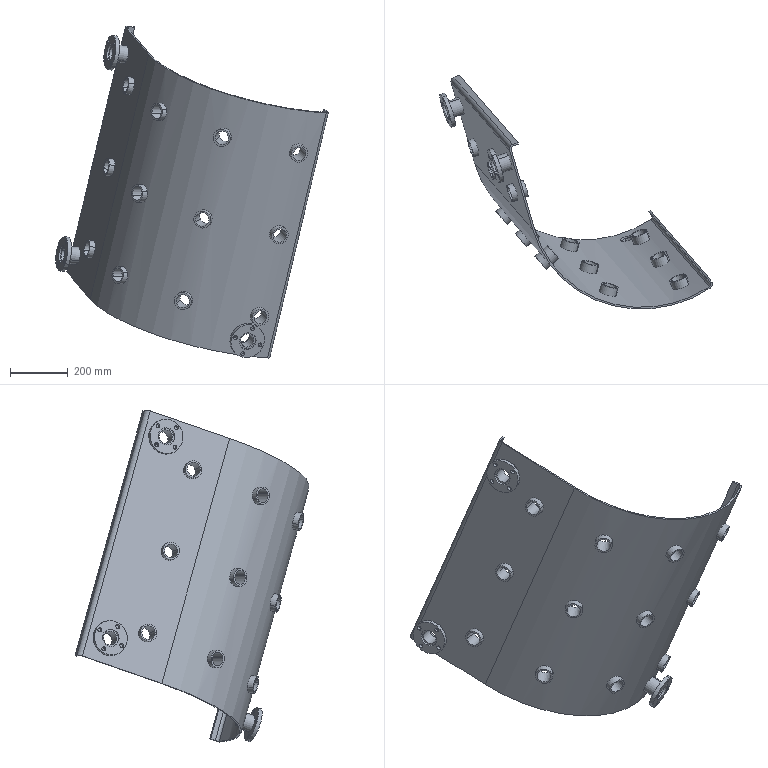Part | SolidWorks | features ReferencePattern 10, LocalLPattern 2, AEMSimFeature 1, LocalCirPattern 1, MirrorCompFeat 1 | 19 solids | 188 faces | box 940.727 x 808.112 x 1146 mm | volume 7168589 mm3 | cylinder 132 | plane 56 | commonest cylinder face diameters 60 x60 48 x34 14 x24 120 x6 20 x2 32 x2